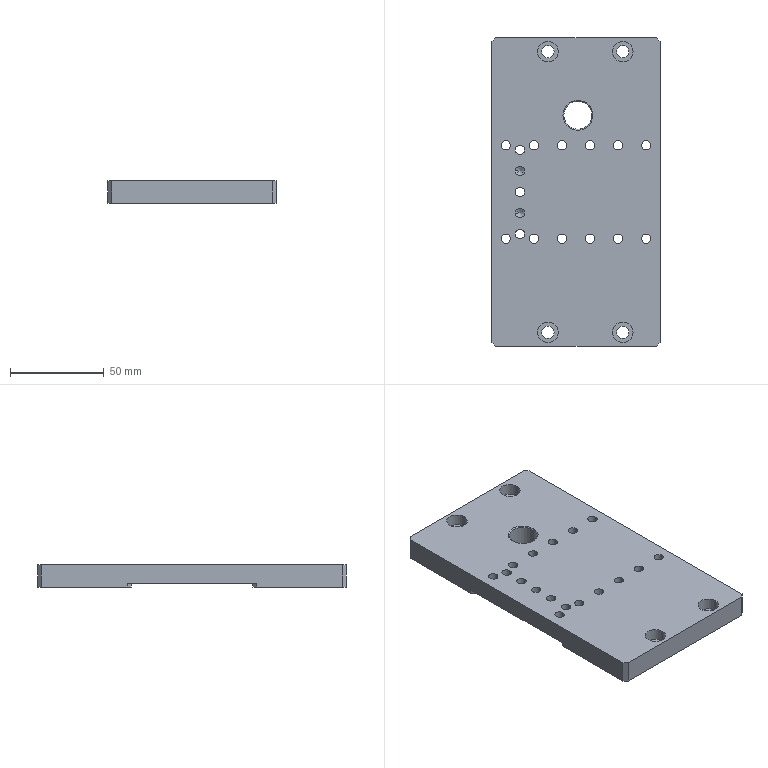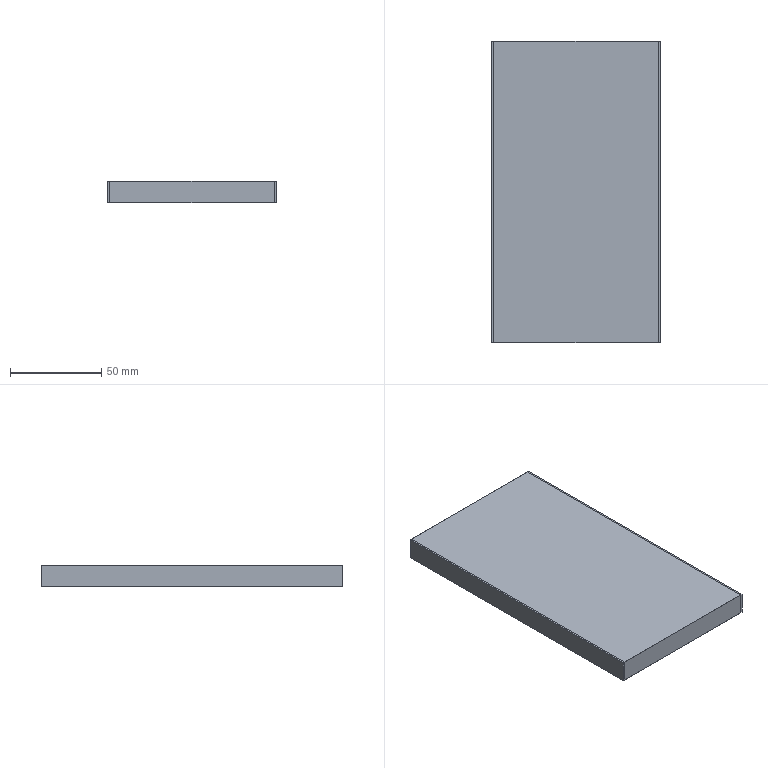CAM job | NX | 3-axis milling, drilling | part box 90 x 165 x 12 mm | stock box 92 x 165 x 12 mm
Tools:
number,name,description,diameter,corner_radius,flute_length,length,flutes
15,D10,Milling Tool-5 Parameters,10.0,0.0,50.0,75.0,2
14,D10JING,Milling Tool-5 Parameters,10.0,0.0,50.0,75.0,2
1,D6A45,Milling Tool-5 Parameters,6.0,0.0,50.0,75.0,2
10,6.6ZT,Drilling Tool,6.6,0.0,35.0,50.0,2
17,5.0ZT,Drilling Tool,5.0,0.0,35.0,50.0,2
12,D6,Milling Tool-5 Parameters,6.0,0.0,50.0,75.0,2
18,D3,Milling Tool-5 Parameters,3.0,0.0,50.0,75.0,2
Operations:
program,operation,operation_type,tool,method,geometry_group,spindle_rpm,surface_speed,feed_per_tooth,feed_cut,feed_plunge,cut_length_mm,path_length_mm,cut_time_min,machine_time_min
1,DRILLING,Operation,D6A45,METHOD,A,9500.0,179.0,0.0132,250.0,0.0,88.0,714.453,0.352,0.4146
1,DRILLING_COPY,Operation,6.6ZT,METHOD,A,2000.0,41.0,0.0625,250.0,0.0,69.931,439.117,0.2797,0.3166
1,DRILLING_COPY_COPY,Operation,5.0ZT,METHOD,A,2000.0,41.0,0.0625,250.0,0.0,255.032,820.809,1.02,1.077
1,ZLEVEL_PROFILE,ZLevelMilling,D10,METHOD,A,9500.0,298.0,0.1579,3000.0,1000.0,2915.764,3323.552,1.062,1.103
1,HOLE_MILLING,CylinderMilling,D6,METHOD,A,9500.0,179.0,0.0789,1500.0,100.0,1764.929,2348.562,1.177,1.235
1,HOLE_MILLING_COPY,CylinderMilling,D3,METHOD,A,9500.0,89.0,0.0632,1200.0,100.0,384.761,538.261,0.3206,0.336
1,ZLEVEL_PROFILE_1,ZLevelMilling,D10JING,METHOD,A,9500.0,298.0,0.0789,1500.0,1000.0,215.259,545.595,0.1462,0.1792
1,PLANAR_MILL_COPY,PlanarMilling,D6A45,METHOD,A,9500.0,179.0,0.0658,1250.0,100.0,909.558,2699.075,0.7276,0.9066
1,PLANAR_MILL_COPY_COPY,PlanarMilling,D6A45,METHOD,A,9500.0,179.0,0.0658,1250.0,100.0,45.935,105.935,0.0367,0.0427
1,18刀补,CylinderMilling,D3,METHOD,A,9500.0,89.0,0.0632,1200.0,100.0,58.867,212.367,0.0491,0.0644
2,FLOOR_WALL_1,VolumeBased25DMillingOperation,D10,METHOD,B,9500.0,298.0,0.1842,3500.0,1000.0,2634.172,2720.142,0.7579,0.7665
2,FLOOR_WALL_1_COPY,VolumeBased25DMillingOperation,D10JING,METHOD,B,9500.0,298.0,0.0789,1500.0,1000.0,1482.206,1615.386,0.9915,1.005
2,PLANAR_MILL_COPY_COPY_1,PlanarMilling,D6A45,METHOD,B,9500.0,179.0,0.0658,1250.0,100.0,652.756,1284.198,0.5222,0.5853
2,PLANAR_MILL_COPY_COPY_COPY,PlanarMilling,D6A45,METHOD,B,9500.0,179.0,0.0658,1250.0,100.0,45.935,105.935,0.0367,0.0427
2,PLANAR_MILL_COPY_COPY_1_COPY,PlanarMilling,D6A45,METHOD,B,9500.0,179.0,0.0658,1250.0,100.0,392.435,1860.845,0.3139,0.4608